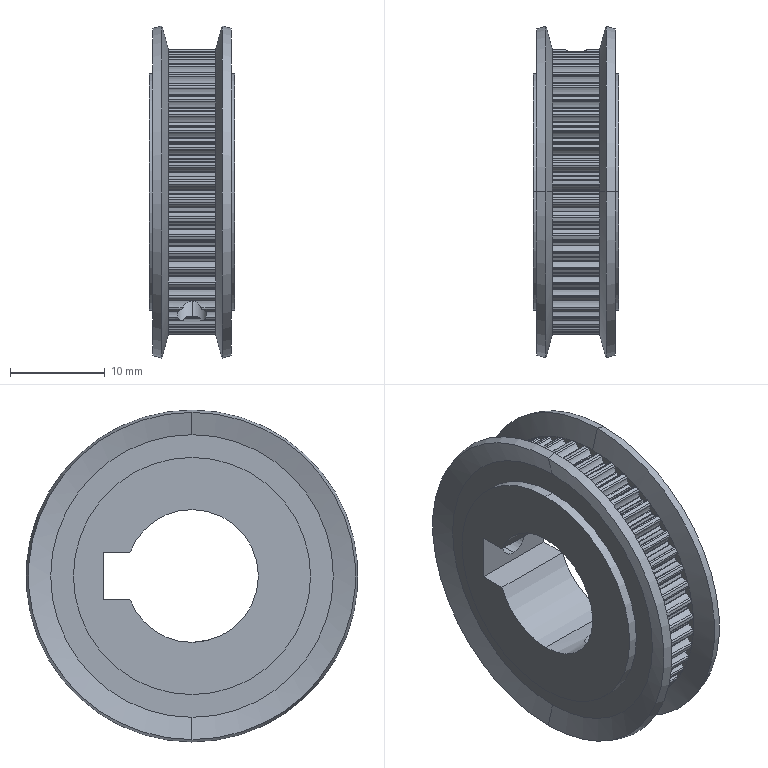Part | SolidWorks | features BaseBody 1 | 1 solid | 574 faces | box 9 x 35 x 35 mm | volume 4657 mm3 | cylinder 459 | plane 103 | cone 12 | commonest cylinder face diameters 0.38 x124 0.2 x113 2.65 x108 30.05 x52 28.53 x51 3.242 x4